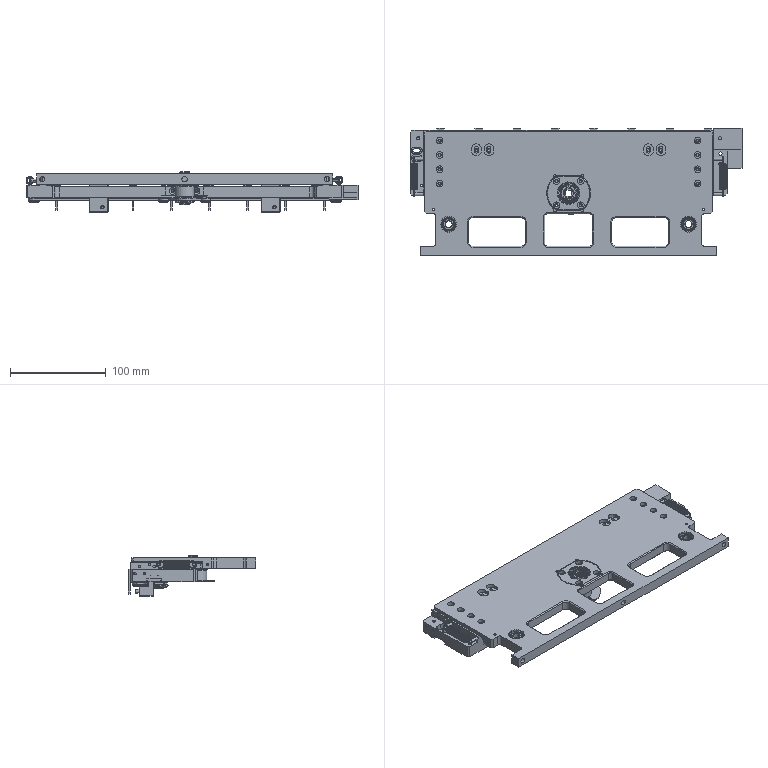Part | NX | features BREP 29 | 60 solids | 3045 faces | volume 467322 mm3 | plane 1168 | cylinder 1144 | sphere 272 | cone 241 | torus 154 | spline 66 | commonest cylinder face diameters 0.46 x120 4 x111 2.5 x104 6 x90 3.4 x84 10 x84